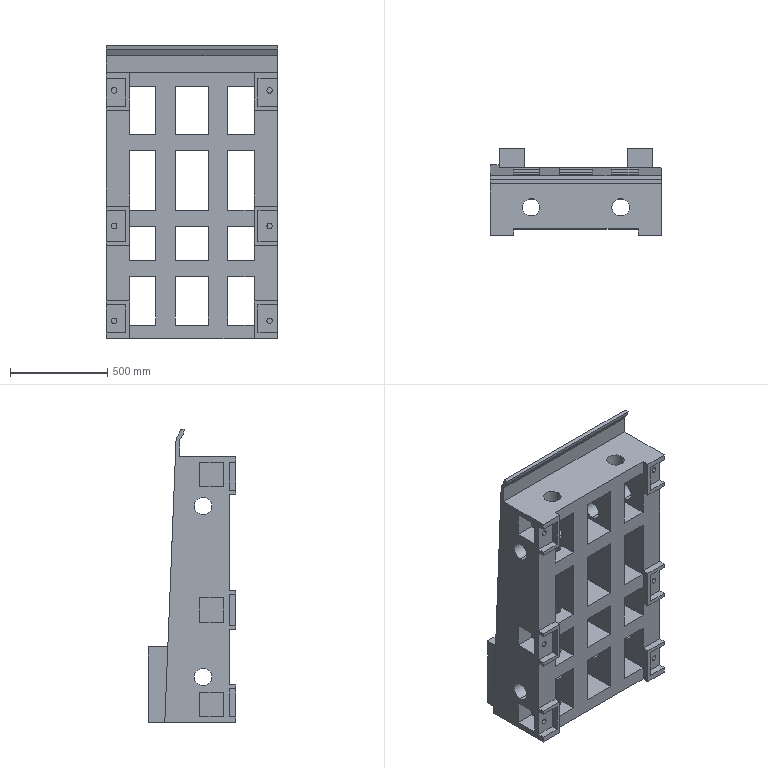Part | STEP file | M20 Tapped Hole 3 | 1 solid | 211 faces | box 880.9 x 451 x 1510 mm | volume 224159075 mm3 | plane 139 | cylinder 60 | cone 12 | commonest cylinder face diameters 90 x36 17.5 x12 28 x12